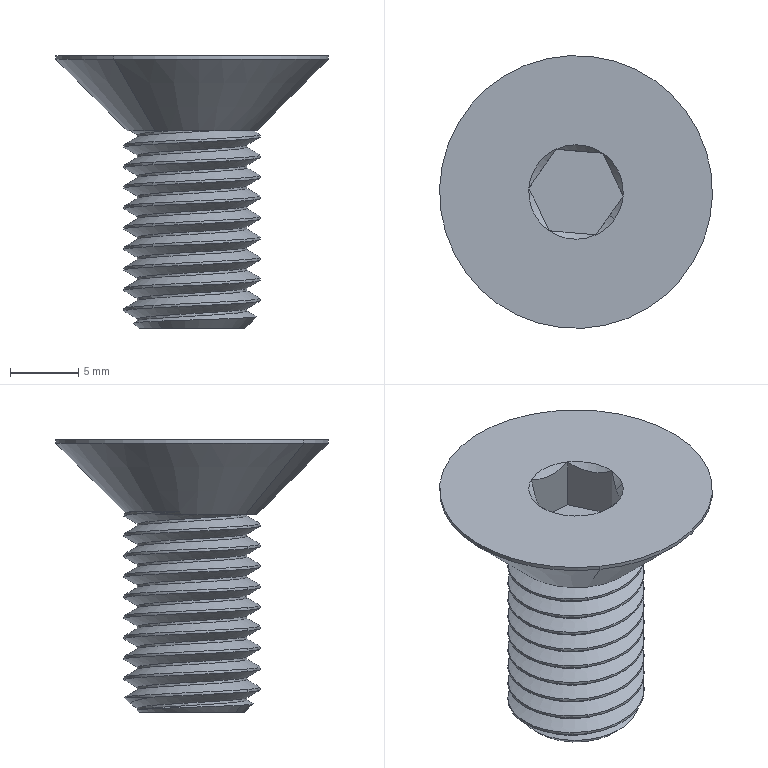Part | NX | features solid 2 | 1 solid | 46 faces | box 20 x 20 x 20 mm | volume 1823 mm3 | cylinder 21 | cone 12 | plane 10 | spline 3 | commonest cylinder face diameters 10 x19 20 x2